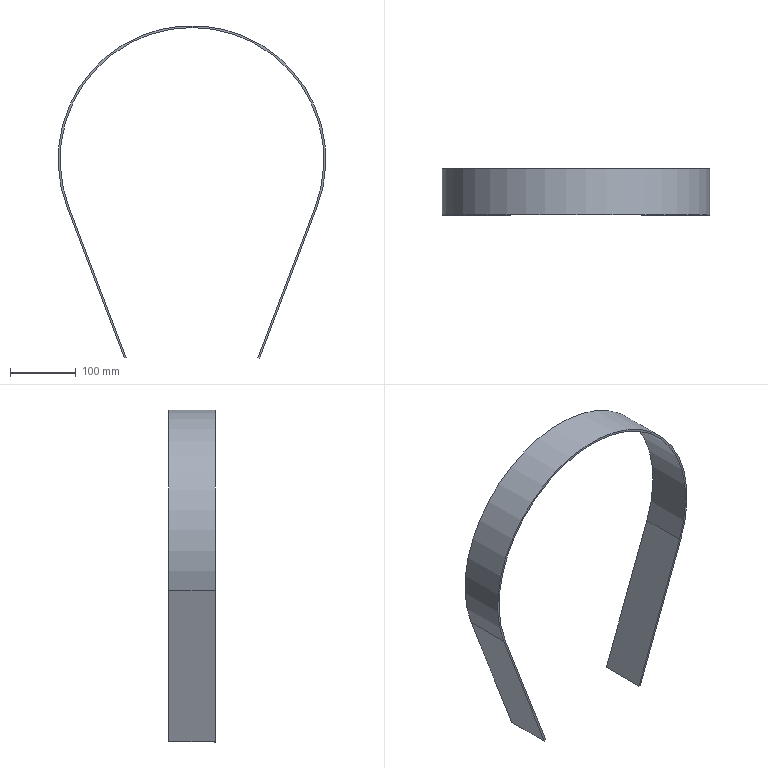Part | SolidWorks | 1 solid | 14 faces | box 406 x 70 x 504.065 mm | volume 266533 mm3 | plane 12 | cylinder 2 | commonest cylinder face diameters 400 x1 406 x1
STEP:
#1=CARTESIAN_POINT('',(102.805,70.,-301.065));
#2=VERTEX_POINT('',#1);
#3=CARTESIAN_POINT('',(102.805,0.,-301.065));
#4=VERTEX_POINT('',#3);
#5=CARTESIAN_POINT('',(102.805,70.,-301.065));
#6=DIRECTION('',(0.,-1.,0.));
#7=VECTOR('',#6,1000.);
#8=LINE('',#5,#7);
#9=EDGE_CURVE('',#2,#4,#8,.T.);
#10=ORIENTED_EDGE('',*,*,#9,.T.);
#11=CARTESIAN_POINT('',(100.,0.,-300.));
#12=VERTEX_POINT('',#11);
#13=CARTESIAN_POINT('',(102.805,0.,-301.065));
#14=DIRECTION('',(-0.9348,0.,0.3551));
#15=VECTOR('',#14,1000.);
#16=LINE('',#13,#15);
#17=EDGE_CURVE('',#4,#12,#16,.T.);
#18=ORIENTED_EDGE('',*,*,#17,.T.);
#19=CARTESIAN_POINT('',(100.,70.,-300.));
#20=VERTEX_POINT('',#19);
#21=CARTESIAN_POINT('',(100.,70.,-300.));
#22=DIRECTION('',(0.,-1.,0.));
#23=VECTOR('',#22,1000.);
#24=LINE('',#21,#23);
#25=EDGE_CURVE('',#20,#12,#24,.T.);
#26=ORIENTED_EDGE('',*,*,#25,.F.);
#27=CARTESIAN_POINT('',(100.,70.,-300.));
#28=DIRECTION('',(0.9348,0.,-0.3551));
#29=VECTOR('',#28,1000.);
#30=LINE('',#27,#29);
#31=EDGE_CURVE('',#20,#2,#30,.T.);
#32=ORIENTED_EDGE('',*,*,#31,.T.);
#33=EDGE_LOOP('',(#10,#18,#26,#32));
#34=FACE_OUTER_BOUND('',#33,.T.);
#35=CARTESIAN_POINT('',(102.805,0.,-301.065));
#36=DIRECTION('',(-0.3551,0.,-0.9348));
#37=DIRECTION('',(-0.9348,0.,0.3551));
#38=AXIS2_PLACEMENT_3D('',#35,#36,#37);
#39=PLANE('',#38);
#40=ADVANCED_FACE('',(#34),#39,.T.);
#41=CARTESIAN_POINT('',(-102.805,70.,-301.065));
#42=VERTEX_POINT('',#41);
#43=CARTESIAN_POINT('',(-102.805,0.,-301.065));
#44=VERTEX_POINT('',#43);
#45=CARTESIAN_POINT('',(-102.805,70.,-301.065));
#46=DIRECTION('',(0.,-1.,0.));
#47=VECTOR('',#46,1000.);
#48=LINE('',#45,#47);
#49=EDGE_CURVE('',#42,#44,#48,.T.);
#50=ORIENTED_EDGE('',*,*,#49,.F.);
#51=CARTESIAN_POINT('',(-100.,70.,-300.));
#52=VERTEX_POINT('',#51);
#53=CARTESIAN_POINT('',(-102.805,70.,-301.065));
#54=DIRECTION('',(0.9348,0.,0.3551));
#55=VECTOR('',#54,1000.);
#56=LINE('',#53,#55);
#57=EDGE_CURVE('',#42,#52,#56,.T.);
#58=ORIENTED_EDGE('',*,*,#57,.T.);
#59=CARTESIAN_POINT('',(-100.,0.,-300.));
#60=VERTEX_POINT('',#59);
#61=CARTESIAN_POINT('',(-100.,0.,-300.));
#62=DIRECTION('',(0.,1.,0.));
#63=VECTOR('',#62,1000.);
#64=LINE('',#61,#63);
#65=EDGE_CURVE('',#60,#52,#64,.T.);
#66=ORIENTED_EDGE('',*,*,#65,.F.);
#67=CARTESIAN_POINT('',(-100.,0.,-300.));
#68=DIRECTION('',(-0.9348,0.,-0.3551));
#69=VECTOR('',#68,1000.);
#70=LINE('',#67,#69);
#71=EDGE_CURVE('',#60,#44,#70,.T.);
#72=ORIENTED_EDGE('',*,*,#71,.T.);
#73=EDGE_LOOP('',(#50,#58,#66,#72));
#74=FACE_OUTER_BOUND('',#73,.T.);
#75=CARTESIAN_POINT('',(-102.805,70.,-301.065));
#76=DIRECTION('',(0.3551,0.,-0.9348));
#77=DIRECTION('',(0.,-1.,0.));
#78=AXIS2_PLACEMENT_3D('',#75,#76,#77);
#79=PLANE('',#78);
#80=ADVANCED_FACE('',(#74),#79,.T.);
#81=ORIENTED_EDGE('',*,*,#57,.F.);
#82=CARTESIAN_POINT('',(-189.774,70.,-72.075));
#83=VERTEX_POINT('',#82);
#84=CARTESIAN_POINT('',(-189.774,70.,-72.075));
#85=DIRECTION('',(0.3551,0.,-0.9348));
#86=VECTOR('',#85,1000.);
#87=LINE('',#84,#86);
#88=EDGE_CURVE('',#83,#42,#87,.T.);
#89=ORIENTED_EDGE('',*,*,#88,.F.);
#90=CARTESIAN_POINT('',(-186.969,70.,-71.01));
#91=VERTEX_POINT('',#90);
#92=CARTESIAN_POINT('',(-189.774,70.,-72.075));
#93=DIRECTION('',(0.9348,0.,0.3551));
#94=VECTOR('',#93,1000.);
#95=LINE('',#92,#94);
#96=EDGE_CURVE('',#83,#91,#95,.T.);
#97=ORIENTED_EDGE('',*,*,#96,.T.);
#98=CARTESIAN_POINT('',(-100.,70.,-300.));
#99=DIRECTION('',(-0.3551,0.,0.9348));
#100=VECTOR('',#99,1000.);
#101=LINE('',#98,#100);
#102=EDGE_CURVE('',#52,#91,#101,.T.);
#103=ORIENTED_EDGE('',*,*,#102,.F.);
#104=EDGE_LOOP('',(#81,#89,#97,#103));
#105=FACE_OUTER_BOUND('',#104,.T.);
#106=CARTESIAN_POINT('',(-189.774,70.,-72.075));
#107=DIRECTION('',(0.,1.,0.));
#108=DIRECTION('',(1.,0.,0.));
#109=AXIS2_PLACEMENT_3D('',#106,#107,#108);
#110=PLANE('',#109);
#111=ADVANCED_FACE('',(#105),#110,.T.);
#112=ORIENTED_EDGE('',*,*,#49,.T.);
#113=CARTESIAN_POINT('',(-189.774,0.,-72.075));
#114=VERTEX_POINT('',#113);
#115=CARTESIAN_POINT('',(-102.805,0.,-301.065));
#116=DIRECTION('',(-0.3551,0.,0.9348));
#117=VECTOR('',#116,1000.);
#118=LINE('',#115,#117);
#119=EDGE_CURVE('',#44,#114,#118,.T.);
#120=ORIENTED_EDGE('',*,*,#119,.T.);
#121=CARTESIAN_POINT('',(-189.774,0.,-72.075));
#122=DIRECTION('',(0.,1.,0.));
#123=VECTOR('',#122,1000.);
#124=LINE('',#121,#123);
#125=EDGE_CURVE('',#114,#83,#124,.T.);
#126=ORIENTED_EDGE('',*,*,#125,.T.);
#127=ORIENTED_EDGE('',*,*,#88,.T.);
#128=EDGE_LOOP('',(#112,#120,#126,#127));
#129=FACE_OUTER_BOUND('',#128,.T.);
#130=CARTESIAN_POINT('',(-327.997,35.,291.866));
#131=DIRECTION('',(0.9348,0.,0.3551));
#132=DIRECTION('',(0.,-1.,0.));
#133=AXIS2_PLACEMENT_3D('',#130,#131,#132);
#134=PLANE('',#133);
#135=ADVANCED_FACE('',(#129),#134,.F.);
#136=ORIENTED_EDGE('',*,*,#71,.F.);
#137=CARTESIAN_POINT('',(-186.969,0.,-71.01));
#138=VERTEX_POINT('',#137);
#139=CARTESIAN_POINT('',(-186.969,0.,-71.01));
#140=DIRECTION('',(0.3551,0.,-0.9348));
#141=VECTOR('',#140,1000.);
#142=LINE('',#139,#141);
#143=EDGE_CURVE('',#138,#60,#142,.T.);
#144=ORIENTED_EDGE('',*,*,#143,.F.);
#145=CARTESIAN_POINT('',(-186.969,0.,-71.01));
#146=DIRECTION('',(-0.9348,0.,-0.3551));
#147=VECTOR('',#146,1000.);
#148=LINE('',#145,#147);
#149=EDGE_CURVE('',#138,#114,#148,.T.);
#150=ORIENTED_EDGE('',*,*,#149,.T.);
#151=ORIENTED_EDGE('',*,*,#119,.F.);
#152=EDGE_LOOP('',(#136,#144,#150,#151));
#153=FACE_OUTER_BOUND('',#152,.T.);
#154=CARTESIAN_POINT('',(-466.221,0.,655.807));
#155=DIRECTION('',(0.,-1.,0.));
#156=DIRECTION('',(0.,0.,-1.));
#157=AXIS2_PLACEMENT_3D('',#154,#155,#156);
#158=PLANE('',#157);
#159=ADVANCED_FACE('',(#153),#158,.T.);
#160=ORIENTED_EDGE('',*,*,#65,.T.);
#161=ORIENTED_EDGE('',*,*,#102,.T.);
#162=CARTESIAN_POINT('',(-186.969,70.,-71.01));
#163=DIRECTION('',(0.,-1.,0.));
#164=VECTOR('',#163,1000.);
#165=LINE('',#162,#164);
#166=EDGE_CURVE('',#91,#138,#165,.T.);
#167=ORIENTED_EDGE('',*,*,#166,.T.);
#168=ORIENTED_EDGE('',*,*,#143,.T.);
#169=EDGE_LOOP('',(#160,#161,#167,#168));
#170=FACE_OUTER_BOUND('',#169,.T.);
#171=CARTESIAN_POINT('',(-325.193,35.,292.931));
#172=DIRECTION('',(0.9348,0.,0.3551));
#173=DIRECTION('',(0.,-1.,0.));
#174=AXIS2_PLACEMENT_3D('',#171,#172,#173);
#175=PLANE('',#174);
#176=ADVANCED_FACE('',(#170),#175,.T.);
#177=CARTESIAN_POINT('',(186.969,0.,-71.01));
#178=VERTEX_POINT('',#177);
#179=CARTESIAN_POINT('',(0.,0.,0.));
#180=DIRECTION('',(0.,-1.,0.));
#181=DIRECTION('',(0.9348,0.,-0.3551));
#182=AXIS2_PLACEMENT_3D('',#179,#180,#181);
#183=CIRCLE('',#182,200.);
#184=EDGE_CURVE('',#178,#138,#183,.T.);
#185=ORIENTED_EDGE('',*,*,#184,.T.);
#186=ORIENTED_EDGE('',*,*,#166,.F.);
#187=CARTESIAN_POINT('',(186.969,70.,-71.01));
#188=VERTEX_POINT('',#187);
#189=CARTESIAN_POINT('',(0.,70.,0.));
#190=DIRECTION('',(0.,1.,0.));
#191=DIRECTION('',(-0.9348,0.,-0.3551));
#192=AXIS2_PLACEMENT_3D('',#189,#190,#191);
#193=CIRCLE('',#192,200.);
#194=EDGE_CURVE('',#91,#188,#193,.T.);
#195=ORIENTED_EDGE('',*,*,#194,.T.);
#196=CARTESIAN_POINT('',(186.969,0.,-71.01));
#197=DIRECTION('',(0.,1.,0.));
#198=VECTOR('',#197,1000.);
#199=LINE('',#196,#198);
#200=EDGE_CURVE('',#178,#188,#199,.T.);
#201=ORIENTED_EDGE('',*,*,#200,.F.);
#202=EDGE_LOOP('',(#185,#186,#195,#201));
#203=FACE_OUTER_BOUND('',#202,.T.);
#204=CARTESIAN_POINT('',(0.,35.,0.));
#205=DIRECTION('',(0.,1.,0.));
#206=DIRECTION('',(-0.9348,0.,-0.3551));
#207=AXIS2_PLACEMENT_3D('',#204,#205,#206);
#208=CYLINDRICAL_SURFACE('',#207,200.);
#209=ADVANCED_FACE('',(#203),#208,.F.);
#210=ORIENTED_EDGE('',*,*,#96,.F.);
#211=CARTESIAN_POINT('',(189.774,70.,-72.075));
#212=VERTEX_POINT('',#211);
#213=CARTESIAN_POINT('',(0.,70.,0.));
#214=DIRECTION('',(0.,-1.,0.));
#215=DIRECTION('',(0.9348,0.,-0.3551));
#216=AXIS2_PLACEMENT_3D('',#213,#214,#215);
#217=CIRCLE('',#216,203.);
#218=EDGE_CURVE('',#212,#83,#217,.T.);
#219=ORIENTED_EDGE('',*,*,#218,.F.);
#220=CARTESIAN_POINT('',(189.774,70.,-72.075));
#221=DIRECTION('',(-0.9348,0.,0.3551));
#222=VECTOR('',#221,1000.);
#223=LINE('',#220,#222);
#224=EDGE_CURVE('',#212,#188,#223,.T.);
#225=ORIENTED_EDGE('',*,*,#224,.T.);
#226=ORIENTED_EDGE('',*,*,#194,.F.);
#227=EDGE_LOOP('',(#210,#219,#225,#226));
#228=FACE_OUTER_BOUND('',#227,.T.);
#229=CARTESIAN_POINT('',(186.969,70.,-71.01));
#230=DIRECTION('',(0.,1.,0.));
#231=DIRECTION('',(1.,0.,0.));
#232=AXIS2_PLACEMENT_3D('',#229,#230,#231);
#233=PLANE('',#232);
#234=ADVANCED_FACE('',(#228),#233,.T.);
#235=ORIENTED_EDGE('',*,*,#218,.T.);
#236=ORIENTED_EDGE('',*,*,#125,.F.);
#237=CARTESIAN_POINT('',(189.774,0.,-72.075));
#238=VERTEX_POINT('',#237);
#239=CARTESIAN_POINT('',(0.,0.,0.));
#240=DIRECTION('',(0.,1.,0.));
#241=DIRECTION('',(-0.9348,0.,-0.3551));
#242=AXIS2_PLACEMENT_3D('',#239,#240,#241);
#243=CIRCLE('',#242,203.);
#244=EDGE_CURVE('',#114,#238,#243,.T.);
#245=ORIENTED_EDGE('',*,*,#244,.T.);
#246=CARTESIAN_POINT('',(189.774,70.,-72.075));
#247=DIRECTION('',(0.,-1.,0.));
#248=VECTOR('',#247,1000.);
#249=LINE('',#246,#248);
#250=EDGE_CURVE('',#212,#238,#249,.T.);
#251=ORIENTED_EDGE('',*,*,#250,.F.);
#252=EDGE_LOOP('',(#235,#236,#245,#251));
#253=FACE_OUTER_BOUND('',#252,.T.);
#254=CARTESIAN_POINT('',(0.,35.,0.));
#255=DIRECTION('',(0.,1.,0.));
#256=DIRECTION('',(-0.9348,0.,-0.3551));
#257=AXIS2_PLACEMENT_3D('',#254,#255,#256);
#258=CYLINDRICAL_SURFACE('',#257,203.);
#259=ADVANCED_FACE('',(#253),#258,.T.);
#260=ORIENTED_EDGE('',*,*,#9,.F.);
#261=CARTESIAN_POINT('',(102.805,70.,-301.065));
#262=DIRECTION('',(0.3551,0.,0.9348));
#263=VECTOR('',#262,1000.);
#264=LINE('',#261,#263);
#265=EDGE_CURVE('',#2,#212,#264,.T.);
#266=ORIENTED_EDGE('',*,*,#265,.T.);
#267=ORIENTED_EDGE('',*,*,#250,.T.);
#268=CARTESIAN_POINT('',(189.774,0.,-72.075));
#269=DIRECTION('',(-0.3551,0.,-0.9348));
#270=VECTOR('',#269,1000.);
#271=LINE('',#268,#270);
#272=EDGE_CURVE('',#238,#4,#271,.T.);
#273=ORIENTED_EDGE('',*,*,#272,.T.);
#274=EDGE_LOOP('',(#260,#266,#267,#273));
#275=FACE_OUTER_BOUND('',#274,.T.);
#276=CARTESIAN_POINT('',(327.997,35.,291.866));
#277=DIRECTION('',(-0.9348,0.,0.3551));
#278=DIRECTION('',(0.,1.,0.));
#279=AXIS2_PLACEMENT_3D('',#276,#277,#278);
#280=PLANE('',#279);
#281=ADVANCED_FACE('',(#275),#280,.F.);
#282=ORIENTED_EDGE('',*,*,#31,.F.);
#283=CARTESIAN_POINT('',(186.969,70.,-71.01));
#284=DIRECTION('',(-0.3551,0.,-0.9348));
#285=VECTOR('',#284,1000.);
#286=LINE('',#283,#285);
#287=EDGE_CURVE('',#188,#20,#286,.T.);
#288=ORIENTED_EDGE('',*,*,#287,.F.);
#289=ORIENTED_EDGE('',*,*,#224,.F.);
#290=ORIENTED_EDGE('',*,*,#265,.F.);
#291=EDGE_LOOP('',(#282,#288,#289,#290));
#292=FACE_OUTER_BOUND('',#291,.T.);
#293=CARTESIAN_POINT('',(466.221,70.,655.807));
#294=DIRECTION('',(0.,1.,0.));
#295=DIRECTION('',(1.,0.,0.));
#296=AXIS2_PLACEMENT_3D('',#293,#294,#295);
#297=PLANE('',#296);
#298=ADVANCED_FACE('',(#292),#297,.T.);
#299=ORIENTED_EDGE('',*,*,#25,.T.);
#300=CARTESIAN_POINT('',(100.,0.,-300.));
#301=DIRECTION('',(0.3551,0.,0.9348));
#302=VECTOR('',#301,1000.);
#303=LINE('',#300,#302);
#304=EDGE_CURVE('',#12,#178,#303,.T.);
#305=ORIENTED_EDGE('',*,*,#304,.T.);
#306=ORIENTED_EDGE('',*,*,#200,.T.);
#307=ORIENTED_EDGE('',*,*,#287,.T.);
#308=EDGE_LOOP('',(#299,#305,#306,#307));
#309=FACE_OUTER_BOUND('',#308,.T.);
#310=CARTESIAN_POINT('',(325.193,35.,292.931));
#311=DIRECTION('',(-0.9348,0.,0.3551));
#312=DIRECTION('',(0.,1.,0.));
#313=AXIS2_PLACEMENT_3D('',#310,#311,#312);
#314=PLANE('',#313);
#315=ADVANCED_FACE('',(#309),#314,.T.);
#316=ORIENTED_EDGE('',*,*,#17,.F.);
#317=ORIENTED_EDGE('',*,*,#272,.F.);
#318=CARTESIAN_POINT('',(186.969,0.,-71.01));
#319=DIRECTION('',(0.9348,0.,-0.3551));
#320=VECTOR('',#319,1000.);
#321=LINE('',#318,#320);
#322=EDGE_CURVE('',#178,#238,#321,.T.);
#323=ORIENTED_EDGE('',*,*,#322,.F.);
#324=ORIENTED_EDGE('',*,*,#304,.F.);
#325=EDGE_LOOP('',(#316,#317,#323,#324));
#326=FACE_OUTER_BOUND('',#325,.T.);
#327=CARTESIAN_POINT('',(189.774,0.,-72.075));
#328=DIRECTION('',(0.,-1.,0.));
#329=DIRECTION('',(0.,0.,-1.));
#330=AXIS2_PLACEMENT_3D('',#327,#328,#329);
#331=PLANE('',#330);
#332=ADVANCED_FACE('',(#326),#331,.T.);
#333=ORIENTED_EDGE('',*,*,#322,.T.);
#334=ORIENTED_EDGE('',*,*,#244,.F.);
#335=ORIENTED_EDGE('',*,*,#149,.F.);
#336=ORIENTED_EDGE('',*,*,#184,.F.);
#337=EDGE_LOOP('',(#333,#334,#335,#336));
#338=FACE_OUTER_BOUND('',#337,.T.);
#339=CARTESIAN_POINT('',(189.774,0.,-72.075));
#340=DIRECTION('',(0.,-1.,0.));
#341=DIRECTION('',(0.,0.,-1.));
#342=AXIS2_PLACEMENT_3D('',#339,#340,#341);
#343=PLANE('',#342);
#344=ADVANCED_FACE('',(#338),#343,.T.);
#345=CLOSED_SHELL('',(#40,#80,#111,#135,#159,#176,#209,#234,#259,#281,#298,#315,#332,#344));
#346=MANIFOLD_SOLID_BREP('',#345);
#347=CARTESIAN_POINT('',(0.,0.,0.));
#348=DIRECTION('',(0.,0.,1.));
#349=DIRECTION('',(1.,0.,0.));
#350=AXIS2_PLACEMENT_3D('',#347,#348,#349);
#351=(LENGTH_UNIT()NAMED_UNIT(*)SI_UNIT(.MILLI.,.METRE.));
#352=UNCERTAINTY_MEASURE_WITH_UNIT(LENGTH_MEASURE(0.00001),#351,'','');
#353=(NAMED_UNIT(*)PLANE_ANGLE_UNIT()SI_UNIT($,.RADIAN.));
#354=(NAMED_UNIT(*)SI_UNIT($,.STERADIAN.)SOLID_ANGLE_UNIT());
#355=(GEOMETRIC_REPRESENTATION_CONTEXT(3)GLOBAL_UNCERTAINTY_ASSIGNED_CONTEXT((#352))GLOBAL_UNIT_ASSIGNED_CONTEXT((#351,#353,#354))REPRESENTATION_CONTEXT('',''));
#356=ADVANCED_BREP_SHAPE_REPRESENTATION('',(#346,#350),#355);